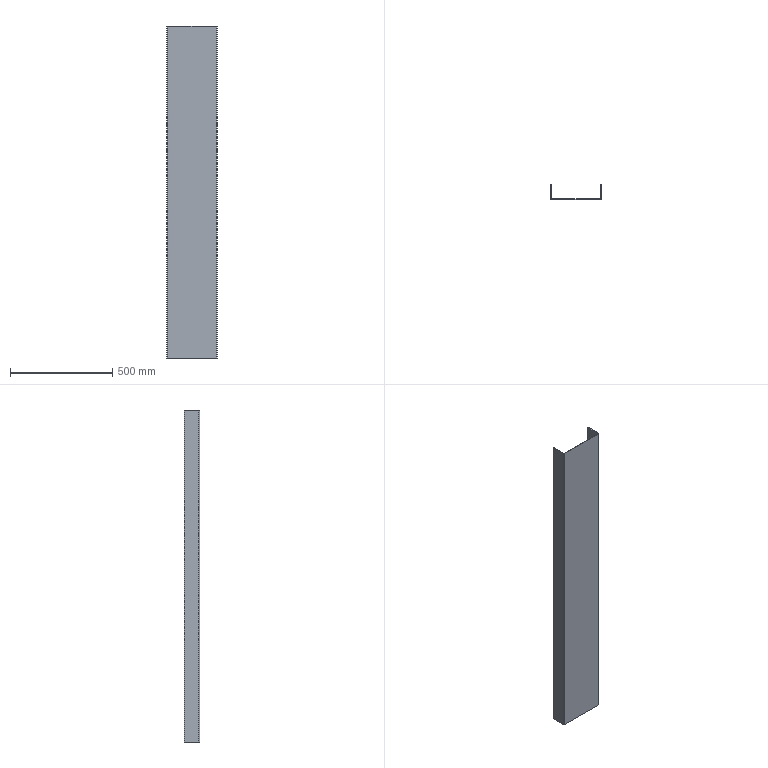Part | STEP file | Sheet metal 12 | 1 solid | 22 faces | box 245 x 75 x 1620 mm | volume 2491073 mm3 | plane 18 | cylinder 4 | commonest cylinder face diameters 2 x2 10 x2
STEP:
#1=CARTESIAN_POINT('',(-117.5,-4.,810.));
#2=VERTEX_POINT('',#1);
#3=CARTESIAN_POINT('',(-117.5,-4.,-810.));
#4=VERTEX_POINT('',#3);
#5=CARTESIAN_POINT('',(-117.5,-4.,810.));
#6=DIRECTION('',(0.,0.,-1.));
#7=VECTOR('',#6,1000.);
#8=LINE('',#5,#7);
#9=EDGE_CURVE('',#2,#4,#8,.T.);
#10=ORIENTED_EDGE('',*,*,#9,.T.);
#11=CARTESIAN_POINT('',(117.5,-4.,-810.));
#12=VERTEX_POINT('',#11);
#13=CARTESIAN_POINT('',(-122.5,-4.,-810.));
#14=DIRECTION('',(-1.,0.,0.));
#15=VECTOR('',#14,1000.);
#16=LINE('',#13,#15);
#17=EDGE_CURVE('',#12,#4,#16,.T.);
#18=ORIENTED_EDGE('',*,*,#17,.F.);
#19=CARTESIAN_POINT('',(117.5,-4.,810.));
#20=VERTEX_POINT('',#19);
#21=CARTESIAN_POINT('',(117.5,-4.,-810.));
#22=DIRECTION('',(0.,0.,1.));
#23=VECTOR('',#22,1000.);
#24=LINE('',#21,#23);
#25=EDGE_CURVE('',#12,#20,#24,.T.);
#26=ORIENTED_EDGE('',*,*,#25,.T.);
#27=CARTESIAN_POINT('',(-122.5,-4.,810.));
#28=DIRECTION('',(1.,0.,0.));
#29=VECTOR('',#28,1000.);
#30=LINE('',#27,#29);
#31=EDGE_CURVE('',#2,#20,#30,.T.);
#32=ORIENTED_EDGE('',*,*,#31,.F.);
#33=EDGE_LOOP('',(#10,#18,#26,#32));
#34=FACE_OUTER_BOUND('',#33,.T.);
#35=CARTESIAN_POINT('',(0.,-4.,0.));
#36=DIRECTION('',(0.,1.,0.));
#37=DIRECTION('',(0.,0.,1.));
#38=AXIS2_PLACEMENT_3D('',#35,#36,#37);
#39=PLANE('',#38);
#40=ADVANCED_FACE('',(#34),#39,.F.);
#41=CARTESIAN_POINT('',(117.5,0.,-810.));
#42=VERTEX_POINT('',#41);
#43=CARTESIAN_POINT('',(-117.5,0.,-810.));
#44=VERTEX_POINT('',#43);
#45=CARTESIAN_POINT('',(-122.5,0.,-810.));
#46=DIRECTION('',(-1.,0.,0.));
#47=VECTOR('',#46,1000.);
#48=LINE('',#45,#47);
#49=EDGE_CURVE('',#42,#44,#48,.T.);
#50=ORIENTED_EDGE('',*,*,#49,.T.);
#51=CARTESIAN_POINT('',(-117.5,0.,810.));
#52=VERTEX_POINT('',#51);
#53=CARTESIAN_POINT('',(-117.5,0.,810.));
#54=DIRECTION('',(0.,0.,-1.));
#55=VECTOR('',#54,1000.);
#56=LINE('',#53,#55);
#57=EDGE_CURVE('',#52,#44,#56,.T.);
#58=ORIENTED_EDGE('',*,*,#57,.F.);
#59=CARTESIAN_POINT('',(117.5,0.,810.));
#60=VERTEX_POINT('',#59);
#61=CARTESIAN_POINT('',(-122.5,0.,810.));
#62=DIRECTION('',(1.,0.,0.));
#63=VECTOR('',#62,1000.);
#64=LINE('',#61,#63);
#65=EDGE_CURVE('',#52,#60,#64,.T.);
#66=ORIENTED_EDGE('',*,*,#65,.T.);
#67=CARTESIAN_POINT('',(117.5,0.,-810.));
#68=DIRECTION('',(0.,0.,1.));
#69=VECTOR('',#68,1000.);
#70=LINE('',#67,#69);
#71=EDGE_CURVE('',#42,#60,#70,.T.);
#72=ORIENTED_EDGE('',*,*,#71,.F.);
#73=EDGE_LOOP('',(#50,#58,#66,#72));
#74=FACE_OUTER_BOUND('',#73,.T.);
#75=CARTESIAN_POINT('',(0.,0.,0.));
#76=DIRECTION('',(0.,1.,0.));
#77=DIRECTION('',(0.,0.,1.));
#78=AXIS2_PLACEMENT_3D('',#75,#76,#77);
#79=PLANE('',#78);
#80=ADVANCED_FACE('',(#74),#79,.T.);
#81=ORIENTED_EDGE('',*,*,#65,.F.);
#82=CARTESIAN_POINT('',(-117.5,0.,810.));
#83=DIRECTION('',(0.,-1.,0.));
#84=VECTOR('',#83,1000.);
#85=LINE('',#82,#84);
#86=EDGE_CURVE('',#52,#2,#85,.T.);
#87=ORIENTED_EDGE('',*,*,#86,.T.);
#88=ORIENTED_EDGE('',*,*,#31,.T.);
#89=CARTESIAN_POINT('',(117.5,0.,810.));
#90=DIRECTION('',(0.,-1.,0.));
#91=VECTOR('',#90,1000.);
#92=LINE('',#89,#91);
#93=EDGE_CURVE('',#60,#20,#92,.T.);
#94=ORIENTED_EDGE('',*,*,#93,.F.);
#95=EDGE_LOOP('',(#81,#87,#88,#94));
#96=FACE_OUTER_BOUND('',#95,.T.);
#97=CARTESIAN_POINT('',(-122.5,-4.,810.));
#98=DIRECTION('',(0.,0.,1.));
#99=DIRECTION('',(1.,0.,0.));
#100=AXIS2_PLACEMENT_3D('',#97,#98,#99);
#101=PLANE('',#100);
#102=ADVANCED_FACE('',(#96),#101,.T.);
#103=CARTESIAN_POINT('',(-117.5,0.,-810.));
#104=DIRECTION('',(0.,-1.,0.));
#105=VECTOR('',#104,1000.);
#106=LINE('',#103,#105);
#107=EDGE_CURVE('',#44,#4,#106,.T.);
#108=ORIENTED_EDGE('',*,*,#107,.F.);
#109=ORIENTED_EDGE('',*,*,#49,.F.);
#110=CARTESIAN_POINT('',(117.5,0.,-810.));
#111=DIRECTION('',(0.,-1.,0.));
#112=VECTOR('',#111,1000.);
#113=LINE('',#110,#112);
#114=EDGE_CURVE('',#42,#12,#113,.T.);
#115=ORIENTED_EDGE('',*,*,#114,.T.);
#116=ORIENTED_EDGE('',*,*,#17,.T.);
#117=EDGE_LOOP('',(#108,#109,#115,#116));
#118=FACE_OUTER_BOUND('',#117,.T.);
#119=CARTESIAN_POINT('',(-122.5,-4.,-810.));
#120=DIRECTION('',(0.,0.,-1.));
#121=DIRECTION('',(-1.,0.,0.));
#122=AXIS2_PLACEMENT_3D('',#119,#120,#121);
#123=PLANE('',#122);
#124=ADVANCED_FACE('',(#118),#123,.T.);
#125=CARTESIAN_POINT('',(118.5,1.,810.));
#126=VERTEX_POINT('',#125);
#127=CARTESIAN_POINT('',(122.5,1.,810.));
#128=VERTEX_POINT('',#127);
#129=CARTESIAN_POINT('',(122.5,1.,810.));
#130=DIRECTION('',(1.,0.,0.));
#131=VECTOR('',#130,1000.);
#132=LINE('',#129,#131);
#133=EDGE_CURVE('',#126,#128,#132,.T.);
#134=ORIENTED_EDGE('',*,*,#133,.F.);
#135=CARTESIAN_POINT('',(117.5,1.,810.));
#136=DIRECTION('',(0.,0.,1.));
#137=DIRECTION('',(-1.,0.,0.));
#138=AXIS2_PLACEMENT_3D('',#135,#136,#137);
#139=CIRCLE('',#138,1.);
#140=EDGE_CURVE('',#60,#126,#139,.T.);
#141=ORIENTED_EDGE('',*,*,#140,.F.);
#142=ORIENTED_EDGE('',*,*,#93,.T.);
#143=CARTESIAN_POINT('',(117.5,1.,810.));
#144=DIRECTION('',(0.,0.,1.));
#145=DIRECTION('',(-1.,0.,0.));
#146=AXIS2_PLACEMENT_3D('',#143,#144,#145);
#147=CIRCLE('',#146,5.);
#148=EDGE_CURVE('',#20,#128,#147,.T.);
#149=ORIENTED_EDGE('',*,*,#148,.T.);
#150=EDGE_LOOP('',(#134,#141,#142,#149));
#151=FACE_OUTER_BOUND('',#150,.T.);
#152=CARTESIAN_POINT('',(117.5,1.,810.));
#153=DIRECTION('',(0.,0.,1.));
#154=DIRECTION('',(1.,0.,0.));
#155=AXIS2_PLACEMENT_3D('',#152,#153,#154);
#156=PLANE('',#155);
#157=ADVANCED_FACE('',(#151),#156,.T.);
#158=CARTESIAN_POINT('',(118.5,1.,-810.));
#159=VERTEX_POINT('',#158);
#160=CARTESIAN_POINT('',(117.5,1.,-810.));
#161=DIRECTION('',(0.,0.,-1.));
#162=DIRECTION('',(-1.,0.,0.));
#163=AXIS2_PLACEMENT_3D('',#160,#161,#162);
#164=CIRCLE('',#163,1.);
#165=EDGE_CURVE('',#159,#42,#164,.T.);
#166=ORIENTED_EDGE('',*,*,#165,.F.);
#167=CARTESIAN_POINT('',(122.5,1.,-810.));
#168=VERTEX_POINT('',#167);
#169=CARTESIAN_POINT('',(118.5,1.,-810.));
#170=DIRECTION('',(1.,0.,0.));
#171=VECTOR('',#170,1000.);
#172=LINE('',#169,#171);
#173=EDGE_CURVE('',#159,#168,#172,.T.);
#174=ORIENTED_EDGE('',*,*,#173,.T.);
#175=CARTESIAN_POINT('',(117.5,1.,-810.));
#176=DIRECTION('',(0.,0.,-1.));
#177=DIRECTION('',(-1.,0.,0.));
#178=AXIS2_PLACEMENT_3D('',#175,#176,#177);
#179=CIRCLE('',#178,5.);
#180=EDGE_CURVE('',#168,#12,#179,.T.);
#181=ORIENTED_EDGE('',*,*,#180,.T.);
#182=ORIENTED_EDGE('',*,*,#114,.F.);
#183=EDGE_LOOP('',(#166,#174,#181,#182));
#184=FACE_OUTER_BOUND('',#183,.T.);
#185=CARTESIAN_POINT('',(117.5,1.,-810.));
#186=DIRECTION('',(0.,0.,1.));
#187=DIRECTION('',(1.,0.,0.));
#188=AXIS2_PLACEMENT_3D('',#185,#186,#187);
#189=PLANE('',#188);
#190=ADVANCED_FACE('',(#184),#189,.F.);
#191=ORIENTED_EDGE('',*,*,#25,.F.);
#192=ORIENTED_EDGE('',*,*,#180,.F.);
#193=CARTESIAN_POINT('',(122.5,1.,0.));
#194=DIRECTION('',(0.,0.,-1.));
#195=VECTOR('',#194,1000.);
#196=LINE('',#193,#195);
#197=EDGE_CURVE('',#128,#168,#196,.T.);
#198=ORIENTED_EDGE('',*,*,#197,.F.);
#199=ORIENTED_EDGE('',*,*,#148,.F.);
#200=EDGE_LOOP('',(#191,#192,#198,#199));
#201=FACE_OUTER_BOUND('',#200,.T.);
#202=CARTESIAN_POINT('',(117.5,1.,-810.));
#203=DIRECTION('',(0.,0.,-1.));
#204=DIRECTION('',(1.,0.,0.));
#205=AXIS2_PLACEMENT_3D('',#202,#203,#204);
#206=CYLINDRICAL_SURFACE('',#205,5.);
#207=ADVANCED_FACE('',(#201),#206,.T.);
#208=ORIENTED_EDGE('',*,*,#71,.T.);
#209=ORIENTED_EDGE('',*,*,#140,.T.);
#210=CARTESIAN_POINT('',(118.5,1.,810.));
#211=DIRECTION('',(0.,0.,-1.));
#212=VECTOR('',#211,1000.);
#213=LINE('',#210,#212);
#214=EDGE_CURVE('',#126,#159,#213,.T.);
#215=ORIENTED_EDGE('',*,*,#214,.T.);
#216=ORIENTED_EDGE('',*,*,#165,.T.);
#217=EDGE_LOOP('',(#208,#209,#215,#216));
#218=FACE_OUTER_BOUND('',#217,.T.);
#219=CARTESIAN_POINT('',(117.5,1.,-810.));
#220=DIRECTION('',(0.,0.,-1.));
#221=DIRECTION('',(1.,0.,0.));
#222=AXIS2_PLACEMENT_3D('',#219,#220,#221);
#223=CYLINDRICAL_SURFACE('',#222,1.);
#224=ADVANCED_FACE('',(#218),#223,.F.);
#225=CARTESIAN_POINT('',(122.5,71.,-810.));
#226=VERTEX_POINT('',#225);
#227=CARTESIAN_POINT('',(122.5,0.,-810.));
#228=DIRECTION('',(0.,-1.,0.));
#229=VECTOR('',#228,1000.);
#230=LINE('',#227,#229);
#231=EDGE_CURVE('',#226,#168,#230,.T.);
#232=ORIENTED_EDGE('',*,*,#231,.T.);
#233=ORIENTED_EDGE('',*,*,#173,.F.);
#234=CARTESIAN_POINT('',(118.5,71.,-810.));
#235=VERTEX_POINT('',#234);
#236=CARTESIAN_POINT('',(118.5,0.,-810.));
#237=DIRECTION('',(0.,-1.,0.));
#238=VECTOR('',#237,1000.);
#239=LINE('',#236,#238);
#240=EDGE_CURVE('',#235,#159,#239,.T.);
#241=ORIENTED_EDGE('',*,*,#240,.F.);
#242=CARTESIAN_POINT('',(122.5,71.,-810.));
#243=DIRECTION('',(-1.,0.,0.));
#244=VECTOR('',#243,1000.);
#245=LINE('',#242,#244);
#246=EDGE_CURVE('',#226,#235,#245,.T.);
#247=ORIENTED_EDGE('',*,*,#246,.F.);
#248=EDGE_LOOP('',(#232,#233,#241,#247));
#249=FACE_OUTER_BOUND('',#248,.T.);
#250=CARTESIAN_POINT('',(122.5,0.,-810.));
#251=DIRECTION('',(0.,0.,-1.));
#252=DIRECTION('',(-1.,0.,0.));
#253=AXIS2_PLACEMENT_3D('',#250,#251,#252);
#254=PLANE('',#253);
#255=ADVANCED_FACE('',(#249),#254,.T.);
#256=CARTESIAN_POINT('',(118.5,71.,810.));
#257=VERTEX_POINT('',#256);
#258=CARTESIAN_POINT('',(118.5,0.,810.));
#259=DIRECTION('',(0.,1.,0.));
#260=VECTOR('',#259,1000.);
#261=LINE('',#258,#260);
#262=EDGE_CURVE('',#126,#257,#261,.T.);
#263=ORIENTED_EDGE('',*,*,#262,.F.);
#264=ORIENTED_EDGE('',*,*,#133,.T.);
#265=CARTESIAN_POINT('',(122.5,71.,810.));
#266=VERTEX_POINT('',#265);
#267=CARTESIAN_POINT('',(122.5,71.,810.));
#268=DIRECTION('',(0.,1.,0.));
#269=VECTOR('',#268,1000.);
#270=LINE('',#267,#269);
#271=EDGE_CURVE('',#128,#266,#270,.T.);
#272=ORIENTED_EDGE('',*,*,#271,.T.);
#273=CARTESIAN_POINT('',(122.5,71.,810.));
#274=DIRECTION('',(-1.,0.,0.));
#275=VECTOR('',#274,1000.);
#276=LINE('',#273,#275);
#277=EDGE_CURVE('',#266,#257,#276,.T.);
#278=ORIENTED_EDGE('',*,*,#277,.T.);
#279=EDGE_LOOP('',(#263,#264,#272,#278));
#280=FACE_OUTER_BOUND('',#279,.T.);
#281=CARTESIAN_POINT('',(122.5,71.,810.));
#282=DIRECTION('',(0.,0.,1.));
#283=DIRECTION('',(1.,0.,0.));
#284=AXIS2_PLACEMENT_3D('',#281,#282,#283);
#285=PLANE('',#284);
#286=ADVANCED_FACE('',(#280),#285,.T.);
#287=ORIENTED_EDGE('',*,*,#271,.F.);
#288=ORIENTED_EDGE('',*,*,#197,.T.);
#289=ORIENTED_EDGE('',*,*,#231,.F.);
#290=CARTESIAN_POINT('',(122.5,71.,-810.));
#291=DIRECTION('',(0.,0.,-1.));
#292=VECTOR('',#291,1000.);
#293=LINE('',#290,#292);
#294=EDGE_CURVE('',#266,#226,#293,.T.);
#295=ORIENTED_EDGE('',*,*,#294,.F.);
#296=EDGE_LOOP('',(#287,#288,#289,#295));
#297=FACE_OUTER_BOUND('',#296,.T.);
#298=CARTESIAN_POINT('',(122.5,0.,0.));
#299=DIRECTION('',(1.,0.,0.));
#300=DIRECTION('',(0.,1.,0.));
#301=AXIS2_PLACEMENT_3D('',#298,#299,#300);
#302=PLANE('',#301);
#303=ADVANCED_FACE('',(#297),#302,.T.);
#304=ORIENTED_EDGE('',*,*,#214,.F.);
#305=ORIENTED_EDGE('',*,*,#262,.T.);
#306=CARTESIAN_POINT('',(118.5,71.,0.));
#307=DIRECTION('',(0.,0.,-1.));
#308=VECTOR('',#307,1000.);
#309=LINE('',#306,#308);
#310=EDGE_CURVE('',#257,#235,#309,.T.);
#311=ORIENTED_EDGE('',*,*,#310,.T.);
#312=ORIENTED_EDGE('',*,*,#240,.T.);
#313=EDGE_LOOP('',(#304,#305,#311,#312));
#314=FACE_OUTER_BOUND('',#313,.T.);
#315=CARTESIAN_POINT('',(118.5,0.,0.));
#316=DIRECTION('',(1.,0.,0.));
#317=DIRECTION('',(0.,1.,0.));
#318=AXIS2_PLACEMENT_3D('',#315,#316,#317);
#319=PLANE('',#318);
#320=ADVANCED_FACE('',(#314),#319,.F.);
#321=ORIENTED_EDGE('',*,*,#310,.F.);
#322=ORIENTED_EDGE('',*,*,#277,.F.);
#323=ORIENTED_EDGE('',*,*,#294,.T.);
#324=ORIENTED_EDGE('',*,*,#246,.T.);
#325=EDGE_LOOP('',(#321,#322,#323,#324));
#326=FACE_OUTER_BOUND('',#325,.T.);
#327=CARTESIAN_POINT('',(122.5,71.,-810.));
#328=DIRECTION('',(0.,1.,0.));
#329=DIRECTION('',(-1.,0.,0.));
#330=AXIS2_PLACEMENT_3D('',#327,#328,#329);
#331=PLANE('',#330);
#332=ADVANCED_FACE('',(#326),#331,.T.);
#333=CARTESIAN_POINT('',(-118.5,1.,-810.));
#334=VERTEX_POINT('',#333);
#335=CARTESIAN_POINT('',(-122.5,1.,-810.));
#336=VERTEX_POINT('',#335);
#337=CARTESIAN_POINT('',(-122.5,1.,-810.));
#338=DIRECTION('',(-1.,0.,0.));
#339=VECTOR('',#338,1000.);
#340=LINE('',#337,#339);
#341=EDGE_CURVE('',#334,#336,#340,.T.);
#342=ORIENTED_EDGE('',*,*,#341,.F.);
#343=CARTESIAN_POINT('',(-117.5,1.,-810.));
#344=DIRECTION('',(0.,0.,-1.));
#345=DIRECTION('',(1.,0.,0.));
#346=AXIS2_PLACEMENT_3D('',#343,#344,#345);
#347=CIRCLE('',#346,1.);
#348=EDGE_CURVE('',#44,#334,#347,.T.);
#349=ORIENTED_EDGE('',*,*,#348,.F.);
#350=ORIENTED_EDGE('',*,*,#107,.T.);
#351=CARTESIAN_POINT('',(-117.5,1.,-810.));
#352=DIRECTION('',(0.,0.,-1.));
#353=DIRECTION('',(1.,0.,0.));
#354=AXIS2_PLACEMENT_3D('',#351,#352,#353);
#355=CIRCLE('',#354,5.);
#356=EDGE_CURVE('',#4,#336,#355,.T.);
#357=ORIENTED_EDGE('',*,*,#356,.T.);
#358=EDGE_LOOP('',(#342,#349,#350,#357));
#359=FACE_OUTER_BOUND('',#358,.T.);
#360=CARTESIAN_POINT('',(-117.5,1.,-810.));
#361=DIRECTION('',(0.,0.,-1.));
#362=DIRECTION('',(-1.,0.,0.));
#363=AXIS2_PLACEMENT_3D('',#360,#361,#362);
#364=PLANE('',#363);
#365=ADVANCED_FACE('',(#359),#364,.T.);
#366=CARTESIAN_POINT('',(-118.5,1.,810.));
#367=VERTEX_POINT('',#366);
#368=CARTESIAN_POINT('',(-117.5,1.,810.));
#369=DIRECTION('',(0.,0.,1.));
#370=DIRECTION('',(1.,0.,0.));
#371=AXIS2_PLACEMENT_3D('',#368,#369,#370);
#372=CIRCLE('',#371,1.);
#373=EDGE_CURVE('',#367,#52,#372,.T.);
#374=ORIENTED_EDGE('',*,*,#373,.F.);
#375=CARTESIAN_POINT('',(-122.5,1.,810.));
#376=VERTEX_POINT('',#375);
#377=CARTESIAN_POINT('',(-118.5,1.,810.));
#378=DIRECTION('',(-1.,0.,0.));
#379=VECTOR('',#378,1000.);
#380=LINE('',#377,#379);
#381=EDGE_CURVE('',#367,#376,#380,.T.);
#382=ORIENTED_EDGE('',*,*,#381,.T.);
#383=CARTESIAN_POINT('',(-117.5,1.,810.));
#384=DIRECTION('',(0.,0.,1.));
#385=DIRECTION('',(1.,0.,0.));
#386=AXIS2_PLACEMENT_3D('',#383,#384,#385);
#387=CIRCLE('',#386,5.);
#388=EDGE_CURVE('',#376,#2,#387,.T.);
#389=ORIENTED_EDGE('',*,*,#388,.T.);
#390=ORIENTED_EDGE('',*,*,#86,.F.);
#391=EDGE_LOOP('',(#374,#382,#389,#390));
#392=FACE_OUTER_BOUND('',#391,.T.);
#393=CARTESIAN_POINT('',(-117.5,1.,810.));
#394=DIRECTION('',(0.,0.,-1.));
#395=DIRECTION('',(-1.,0.,0.));
#396=AXIS2_PLACEMENT_3D('',#393,#394,#395);
#397=PLANE('',#396);
#398=ADVANCED_FACE('',(#392),#397,.F.);
#399=ORIENTED_EDGE('',*,*,#9,.F.);
#400=ORIENTED_EDGE('',*,*,#388,.F.);
#401=CARTESIAN_POINT('',(-122.5,1.,-810.));
#402=DIRECTION('',(0.,0.,-1.));
#403=VECTOR('',#402,1000.);
#404=LINE('',#401,#403);
#405=EDGE_CURVE('',#376,#336,#404,.T.);
#406=ORIENTED_EDGE('',*,*,#405,.T.);
#407=ORIENTED_EDGE('',*,*,#356,.F.);
#408=EDGE_LOOP('',(#399,#400,#406,#407));
#409=FACE_OUTER_BOUND('',#408,.T.);
#410=CARTESIAN_POINT('',(-117.5,1.,810.));
#411=DIRECTION('',(0.,0.,1.));
#412=DIRECTION('',(-1.,0.,0.));
#413=AXIS2_PLACEMENT_3D('',#410,#411,#412);
#414=CYLINDRICAL_SURFACE('',#413,5.);
#415=ADVANCED_FACE('',(#409),#414,.T.);
#416=ORIENTED_EDGE('',*,*,#57,.T.);
#417=ORIENTED_EDGE('',*,*,#348,.T.);
#418=CARTESIAN_POINT('',(-118.5,1.,-810.));
#419=DIRECTION('',(0.,0.,1.));
#420=VECTOR('',#419,1000.);
#421=LINE('',#418,#420);
#422=EDGE_CURVE('',#334,#367,#421,.T.);
#423=ORIENTED_EDGE('',*,*,#422,.T.);
#424=ORIENTED_EDGE('',*,*,#373,.T.);
#425=EDGE_LOOP('',(#416,#417,#423,#424));
#426=FACE_OUTER_BOUND('',#425,.T.);
#427=CARTESIAN_POINT('',(-117.5,1.,810.));
#428=DIRECTION('',(0.,0.,1.));
#429=DIRECTION('',(-1.,0.,0.));
#430=AXIS2_PLACEMENT_3D('',#427,#428,#429);
#431=CYLINDRICAL_SURFACE('',#430,1.);
#432=ADVANCED_FACE('',(#426),#431,.F.);
#433=CARTESIAN_POINT('',(-118.5,71.,-810.));
#434=VERTEX_POINT('',#433);
#435=CARTESIAN_POINT('',(-118.5,0.,-810.));
#436=DIRECTION('',(0.,1.,0.));
#437=VECTOR('',#436,1000.);
#438=LINE('',#435,#437);
#439=EDGE_CURVE('',#334,#434,#438,.T.);
#440=ORIENTED_EDGE('',*,*,#439,.F.);
#441=ORIENTED_EDGE('',*,*,#341,.T.);
#442=CARTESIAN_POINT('',(-122.5,71.,-810.));
#443=VERTEX_POINT('',#442);
#444=CARTESIAN_POINT('',(-122.5,0.,-810.));
#445=DIRECTION('',(0.,1.,0.));
#446=VECTOR('',#445,1000.);
#447=LINE('',#444,#446);
#448=EDGE_CURVE('',#336,#443,#447,.T.);
#449=ORIENTED_EDGE('',*,*,#448,.T.);
#450=CARTESIAN_POINT('',(-122.5,71.,-810.));
#451=DIRECTION('',(1.,0.,0.));
#452=VECTOR('',#451,1000.);
#453=LINE('',#450,#452);
#454=EDGE_CURVE('',#443,#434,#453,.T.);
#455=ORIENTED_EDGE('',*,*,#454,.T.);
#456=EDGE_LOOP('',(#440,#441,#449,#455));
#457=FACE_OUTER_BOUND('',#456,.T.);
#458=CARTESIAN_POINT('',(-122.5,0.,-810.));
#459=DIRECTION('',(0.,0.,-1.));
#460=DIRECTION('',(-1.,0.,0.));
#461=AXIS2_PLACEMENT_3D('',#458,#459,#460);
#462=PLANE('',#461);
#463=ADVANCED_FACE('',(#457),#462,.T.);
#464=CARTESIAN_POINT('',(-122.5,71.,810.));
#465=VERTEX_POINT('',#464);
#466=CARTESIAN_POINT('',(-122.5,71.,810.));
#467=DIRECTION('',(0.,-1.,0.));
#468=VECTOR('',#467,1000.);
#469=LINE('',#466,#468);
#470=EDGE_CURVE('',#465,#376,#469,.T.);
#471=ORIENTED_EDGE('',*,*,#470,.T.);
#472=ORIENTED_EDGE('',*,*,#381,.F.);
#473=CARTESIAN_POINT('',(-118.5,71.,810.));
#474=VERTEX_POINT('',#473);
#475=CARTESIAN_POINT('',(-118.5,0.,810.));
#476=DIRECTION('',(0.,-1.,0.));
#477=VECTOR('',#476,1000.);
#478=LINE('',#475,#477);
#479=EDGE_CURVE('',#474,#367,#478,.T.);
#480=ORIENTED_EDGE('',*,*,#479,.F.);
#481=CARTESIAN_POINT('',(-122.5,71.,810.));
#482=DIRECTION('',(1.,0.,0.));
#483=VECTOR('',#482,1000.);
#484=LINE('',#481,#483);
#485=EDGE_CURVE('',#465,#474,#484,.T.);
#486=ORIENTED_EDGE('',*,*,#485,.F.);
#487=EDGE_LOOP('',(#471,#472,#480,#486));
#488=FACE_OUTER_BOUND('',#487,.T.);
#489=CARTESIAN_POINT('',(-122.5,71.,810.));
#490=DIRECTION('',(0.,0.,1.));
#491=DIRECTION('',(1.,0.,0.));
#492=AXIS2_PLACEMENT_3D('',#489,#490,#491);
#493=PLANE('',#492);
#494=ADVANCED_FACE('',(#488),#493,.T.);
#495=ORIENTED_EDGE('',*,*,#405,.F.);
#496=ORIENTED_EDGE('',*,*,#470,.F.);
#497=CARTESIAN_POINT('',(-122.5,71.,-810.));
#498=DIRECTION('',(0.,0.,1.));
#499=VECTOR('',#498,1000.);
#500=LINE('',#497,#499);
#501=EDGE_CURVE('',#443,#465,#500,.T.);
#502=ORIENTED_EDGE('',*,*,#501,.F.);
#503=ORIENTED_EDGE('',*,*,#448,.F.);
#504=EDGE_LOOP('',(#495,#496,#502,#503));
#505=FACE_OUTER_BOUND('',#504,.T.);
#506=CARTESIAN_POINT('',(-122.5,0.,0.));
#507=DIRECTION('',(1.,0.,0.));
#508=DIRECTION('',(0.,1.,0.));
#509=AXIS2_PLACEMENT_3D('',#506,#507,#508);
#510=PLANE('',#509);
#511=ADVANCED_FACE('',(#505),#510,.F.);
#512=ORIENTED_EDGE('',*,*,#479,.T.);
#513=ORIENTED_EDGE('',*,*,#422,.F.);
#514=ORIENTED_EDGE('',*,*,#439,.T.);
#515=CARTESIAN_POINT('',(-118.5,71.,0.));
#516=DIRECTION('',(0.,0.,1.));
#517=VECTOR('',#516,1000.);
#518=LINE('',#515,#517);
#519=EDGE_CURVE('',#434,#474,#518,.T.);
#520=ORIENTED_EDGE('',*,*,#519,.T.);
#521=EDGE_LOOP('',(#512,#513,#514,#520));
#522=FACE_OUTER_BOUND('',#521,.T.);
#523=CARTESIAN_POINT('',(-118.5,0.,0.));
#524=DIRECTION('',(1.,0.,0.));
#525=DIRECTION('',(0.,1.,0.));
#526=AXIS2_PLACEMENT_3D('',#523,#524,#525);
#527=PLANE('',#526);
#528=ADVANCED_FACE('',(#522),#527,.T.);
#529=ORIENTED_EDGE('',*,*,#519,.F.);
#530=ORIENTED_EDGE('',*,*,#454,.F.);
#531=ORIENTED_EDGE('',*,*,#501,.T.);
#532=ORIENTED_EDGE('',*,*,#485,.T.);
#533=EDGE_LOOP('',(#529,#530,#531,#532));
#534=FACE_OUTER_BOUND('',#533,.T.);
#535=CARTESIAN_POINT('',(-122.5,71.,-810.));
#536=DIRECTION('',(0.,1.,0.));
#537=DIRECTION('',(-1.,0.,0.));
#538=AXIS2_PLACEMENT_3D('',#535,#536,#537);
#539=PLANE('',#538);
#540=ADVANCED_FACE('',(#534),#539,.T.);
#541=CLOSED_SHELL('',(#40,#80,#102,#124,#157,#190,#207,#224,#255,#286,#303,#320,#332,#365,#398,#415,#432,#463,#494,#511,#528,#540));
#542=MANIFOLD_SOLID_BREP('',#541);
#543=CARTESIAN_POINT('',(0.,0.,0.));
#544=DIRECTION('',(0.,0.,1.));
#545=DIRECTION('',(1.,0.,0.));
#546=AXIS2_PLACEMENT_3D('',#543,#544,#545);
#547=(LENGTH_UNIT()NAMED_UNIT(*)SI_UNIT(.MILLI.,.METRE.));
#548=UNCERTAINTY_MEASURE_WITH_UNIT(LENGTH_MEASURE(0.00001),#547,'','');
#549=(NAMED_UNIT(*)PLANE_ANGLE_UNIT()SI_UNIT($,.RADIAN.));
#550=(NAMED_UNIT(*)SI_UNIT($,.STERADIAN.)SOLID_ANGLE_UNIT());
#551=(GEOMETRIC_REPRESENTATION_CONTEXT(3)GLOBAL_UNCERTAINTY_ASSIGNED_CONTEXT((#548))GLOBAL_UNIT_ASSIGNED_CONTEXT((#547,#549,#550))REPRESENTATION_CONTEXT('',''));
#552=ADVANCED_BREP_SHAPE_REPRESENTATION('',(#542,#546),#551);